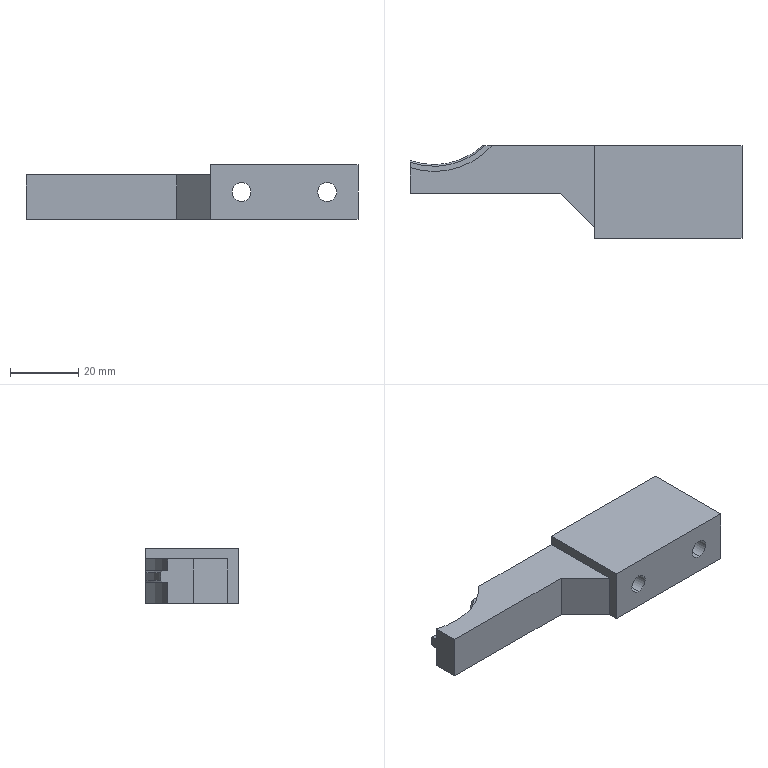Part | SolidWorks | features ICE 9, Chamfer 2, Cut 1, Extrusion 1, Fillet 1, HoleWzd 1, MirrorPattern 1, RefAxis 1 | 1 solid | 27 faces | box 97 x 27 x 16 mm | volume 25539 mm3 | plane 14 | cylinder 11 | cone 2 | commonest cylinder face diameters 5.5 x4 10 x4 46 x2 42 x1
STEP:
#1=CARTESIAN_POINT('',(23.5,14.1,-3.5));
#2=VERTEX_POINT('',#1);
#3=CARTESIAN_POINT('',(23.5,14.1,6.5));
#4=VERTEX_POINT('',#3);
#5=CARTESIAN_POINT('',(23.5,14.1,1.5));
#6=DIRECTION('',(0.,1.,0.));
#7=DIRECTION('',(0.,0.,1.));
#8=AXIS2_PLACEMENT_3D('',#5,#6,#7);
#9=CIRCLE('',#8,5.);
#10=EDGE_CURVE('',#2,#4,#9,.T.);
#11=ORIENTED_EDGE('',*,*,#10,.F.);
#12=CARTESIAN_POINT('',(23.5,19.5,-3.5));
#13=VERTEX_POINT('',#12);
#14=CARTESIAN_POINT('',(23.5,19.5,-3.5));
#15=DIRECTION('',(0.,1.,0.));
#16=VECTOR('',#15,1000.);
#17=LINE('',#14,#16);
#18=EDGE_CURVE('',#2,#13,#17,.T.);
#19=ORIENTED_EDGE('',*,*,#18,.T.);
#20=CARTESIAN_POINT('',(23.5,19.5,6.5));
#21=VERTEX_POINT('',#20);
#22=CARTESIAN_POINT('',(23.5,19.5,1.5));
#23=DIRECTION('',(0.,1.,0.));
#24=DIRECTION('',(0.,0.,1.));
#25=AXIS2_PLACEMENT_3D('',#22,#23,#24);
#26=CIRCLE('',#25,5.);
#27=EDGE_CURVE('',#13,#21,#26,.T.);
#28=ORIENTED_EDGE('',*,*,#27,.T.);
#29=CARTESIAN_POINT('',(23.5,19.5,6.5));
#30=DIRECTION('',(0.,1.,0.));
#31=VECTOR('',#30,1000.);
#32=LINE('',#29,#31);
#33=EDGE_CURVE('',#4,#21,#32,.T.);
#34=ORIENTED_EDGE('',*,*,#33,.F.);
#35=EDGE_LOOP('',(#11,#19,#28,#34));
#36=FACE_OUTER_BOUND('',#35,.T.);
#37=CARTESIAN_POINT('',(23.5,19.5,1.5));
#38=DIRECTION('',(0.,1.,0.));
#39=DIRECTION('',(0.,0.,1.));
#40=AXIS2_PLACEMENT_3D('',#37,#38,#39);
#41=CYLINDRICAL_SURFACE('',#40,5.);
#42=ADVANCED_FACE('',(#36),#41,.F.);
#43=CARTESIAN_POINT('',(23.5,-7.5,-1.25));
#44=VERTEX_POINT('',#43);
#45=CARTESIAN_POINT('',(23.5,-7.5,4.25));
#46=VERTEX_POINT('',#45);
#47=CARTESIAN_POINT('',(23.5,-7.5,1.5));
#48=DIRECTION('',(0.,1.,0.));
#49=DIRECTION('',(0.,0.,1.));
#50=AXIS2_PLACEMENT_3D('',#47,#48,#49);
#51=CIRCLE('',#50,2.75);
#52=EDGE_CURVE('',#44,#46,#51,.T.);
#53=ORIENTED_EDGE('',*,*,#52,.F.);
#54=CARTESIAN_POINT('',(23.5,14.1,-1.25));
#55=VERTEX_POINT('',#54);
#56=CARTESIAN_POINT('',(23.5,19.5,-1.25));
#57=DIRECTION('',(0.,1.,0.));
#58=VECTOR('',#57,1000.);
#59=LINE('',#56,#58);
#60=EDGE_CURVE('',#44,#55,#59,.T.);
#61=ORIENTED_EDGE('',*,*,#60,.T.);
#62=CARTESIAN_POINT('',(23.5,14.1,4.25));
#63=VERTEX_POINT('',#62);
#64=CARTESIAN_POINT('',(23.5,14.1,1.5));
#65=DIRECTION('',(0.,1.,0.));
#66=DIRECTION('',(0.,0.,1.));
#67=AXIS2_PLACEMENT_3D('',#64,#65,#66);
#68=CIRCLE('',#67,2.75);
#69=EDGE_CURVE('',#55,#63,#68,.T.);
#70=ORIENTED_EDGE('',*,*,#69,.T.);
#71=CARTESIAN_POINT('',(23.5,19.5,4.25));
#72=DIRECTION('',(0.,1.,0.));
#73=VECTOR('',#72,1000.);
#74=LINE('',#71,#73);
#75=EDGE_CURVE('',#46,#63,#74,.T.);
#76=ORIENTED_EDGE('',*,*,#75,.F.);
#77=EDGE_LOOP('',(#53,#61,#70,#76));
#78=FACE_OUTER_BOUND('',#77,.T.);
#79=CARTESIAN_POINT('',(23.5,19.5,1.5));
#80=DIRECTION('',(0.,1.,0.));
#81=DIRECTION('',(0.,0.,1.));
#82=AXIS2_PLACEMENT_3D('',#79,#80,#81);
#83=CYLINDRICAL_SURFACE('',#82,2.75);
#84=ADVANCED_FACE('',(#78),#83,.F.);
#85=CARTESIAN_POINT('',(48.5,14.1,-3.5));
#86=VERTEX_POINT('',#85);
#87=CARTESIAN_POINT('',(48.5,14.1,6.5));
#88=VERTEX_POINT('',#87);
#89=CARTESIAN_POINT('',(48.5,14.1,1.5));
#90=DIRECTION('',(0.,1.,0.));
#91=DIRECTION('',(0.,0.,1.));
#92=AXIS2_PLACEMENT_3D('',#89,#90,#91);
#93=CIRCLE('',#92,5.);
#94=EDGE_CURVE('',#86,#88,#93,.T.);
#95=ORIENTED_EDGE('',*,*,#94,.F.);
#96=CARTESIAN_POINT('',(48.5,19.5,-3.5));
#97=VERTEX_POINT('',#96);
#98=CARTESIAN_POINT('',(48.5,19.5,-3.5));
#99=DIRECTION('',(0.,1.,0.));
#100=VECTOR('',#99,1000.);
#101=LINE('',#98,#100);
#102=EDGE_CURVE('',#86,#97,#101,.T.);
#103=ORIENTED_EDGE('',*,*,#102,.T.);
#104=CARTESIAN_POINT('',(48.5,19.5,6.5));
#105=VERTEX_POINT('',#104);
#106=CARTESIAN_POINT('',(48.5,19.5,1.5));
#107=DIRECTION('',(0.,1.,0.));
#108=DIRECTION('',(0.,0.,1.));
#109=AXIS2_PLACEMENT_3D('',#106,#107,#108);
#110=CIRCLE('',#109,5.);
#111=EDGE_CURVE('',#97,#105,#110,.T.);
#112=ORIENTED_EDGE('',*,*,#111,.T.);
#113=CARTESIAN_POINT('',(48.5,19.5,6.5));
#114=DIRECTION('',(0.,1.,0.));
#115=VECTOR('',#114,1000.);
#116=LINE('',#113,#115);
#117=EDGE_CURVE('',#88,#105,#116,.T.);
#118=ORIENTED_EDGE('',*,*,#117,.F.);
#119=EDGE_LOOP('',(#95,#103,#112,#118));
#120=FACE_OUTER_BOUND('',#119,.T.);
#121=CARTESIAN_POINT('',(48.5,19.5,1.5));
#122=DIRECTION('',(0.,1.,0.));
#123=DIRECTION('',(0.,0.,1.));
#124=AXIS2_PLACEMENT_3D('',#121,#122,#123);
#125=CYLINDRICAL_SURFACE('',#124,5.);
#126=ADVANCED_FACE('',(#120),#125,.F.);
#127=CARTESIAN_POINT('',(48.5,-7.5,-1.25));
#128=VERTEX_POINT('',#127);
#129=CARTESIAN_POINT('',(48.5,-7.5,4.25));
#130=VERTEX_POINT('',#129);
#131=CARTESIAN_POINT('',(48.5,-7.5,1.5));
#132=DIRECTION('',(0.,1.,0.));
#133=DIRECTION('',(0.,0.,1.));
#134=AXIS2_PLACEMENT_3D('',#131,#132,#133);
#135=CIRCLE('',#134,2.75);
#136=EDGE_CURVE('',#128,#130,#135,.T.);
#137=ORIENTED_EDGE('',*,*,#136,.F.);
#138=CARTESIAN_POINT('',(48.5,14.1,-1.25));
#139=VERTEX_POINT('',#138);
#140=CARTESIAN_POINT('',(48.5,19.5,-1.25));
#141=DIRECTION('',(0.,1.,0.));
#142=VECTOR('',#141,1000.);
#143=LINE('',#140,#142);
#144=EDGE_CURVE('',#128,#139,#143,.T.);
#145=ORIENTED_EDGE('',*,*,#144,.T.);
#146=CARTESIAN_POINT('',(48.5,14.1,4.25));
#147=VERTEX_POINT('',#146);
#148=CARTESIAN_POINT('',(48.5,14.1,1.5));
#149=DIRECTION('',(0.,1.,0.));
#150=DIRECTION('',(0.,0.,1.));
#151=AXIS2_PLACEMENT_3D('',#148,#149,#150);
#152=CIRCLE('',#151,2.75);
#153=EDGE_CURVE('',#139,#147,#152,.T.);
#154=ORIENTED_EDGE('',*,*,#153,.T.);
#155=CARTESIAN_POINT('',(48.5,19.5,4.25));
#156=DIRECTION('',(0.,1.,0.));
#157=VECTOR('',#156,1000.);
#158=LINE('',#155,#157);
#159=EDGE_CURVE('',#130,#147,#158,.T.);
#160=ORIENTED_EDGE('',*,*,#159,.F.);
#161=EDGE_LOOP('',(#137,#145,#154,#160));
#162=FACE_OUTER_BOUND('',#161,.T.);
#163=CARTESIAN_POINT('',(48.5,19.5,1.5));
#164=DIRECTION('',(0.,1.,0.));
#165=DIRECTION('',(0.,0.,1.));
#166=AXIS2_PLACEMENT_3D('',#163,#164,#165);
#167=CYLINDRICAL_SURFACE('',#166,2.75);
#168=ADVANCED_FACE('',(#162),#167,.F.);
#169=CARTESIAN_POINT('',(23.5,19.5,1.5));
#170=DIRECTION('',(0.,1.,0.));
#171=DIRECTION('',(0.,0.,1.));
#172=AXIS2_PLACEMENT_3D('',#169,#170,#171);
#173=CIRCLE('',#172,5.);
#174=EDGE_CURVE('',#21,#13,#173,.T.);
#175=ORIENTED_EDGE('',*,*,#174,.F.);
#176=ORIENTED_EDGE('',*,*,#27,.F.);
#177=EDGE_LOOP('',(#175,#176));
#178=FACE_BOUND('',#177,.T.);
#179=CARTESIAN_POINT('',(-15.507,19.5,-0.3));
#180=VERTEX_POINT('',#179);
#181=CARTESIAN_POINT('',(-17.6,19.5,-0.3));
#182=VERTEX_POINT('',#181);
#183=CARTESIAN_POINT('',(-32.5,19.5,-0.3));
#184=DIRECTION('',(-1.,0.,0.));
#185=VECTOR('',#184,1000.);
#186=LINE('',#183,#185);
#187=EDGE_CURVE('',#180,#182,#186,.T.);
#188=ORIENTED_EDGE('',*,*,#187,.T.);
#189=CARTESIAN_POINT('',(-18.331,19.5,0.2));
#190=VERTEX_POINT('',#189);
#191=CARTESIAN_POINT('',(-17.6,19.5,-0.3));
#192=CARTESIAN_POINT('',(-17.843,19.5,-0.1317));
#193=CARTESIAN_POINT('',(-18.087,19.5,0.03503));
#194=CARTESIAN_POINT('',(-18.331,19.5,0.2));
#195=B_SPLINE_CURVE_WITH_KNOTS('',3,(#191,#192,#193,#194),.UNSPECIFIED.,.F.,.F.,(4,4),(0.000001215,0.0008778),.UNSPECIFIED.);
#196=EDGE_CURVE('',#182,#190,#195,.T.);
#197=ORIENTED_EDGE('',*,*,#196,.T.);
#198=CARTESIAN_POINT('',(-18.331,19.5,2.5));
#199=VERTEX_POINT('',#198);
#200=CARTESIAN_POINT('',(-18.331,19.5,-9.5));
#201=DIRECTION('',(0.,0.,-1.));
#202=VECTOR('',#201,1000.);
#203=LINE('',#200,#202);
#204=EDGE_CURVE('',#199,#190,#203,.T.);
#205=ORIENTED_EDGE('',*,*,#204,.F.);
#206=CARTESIAN_POINT('',(-17.6,19.5,3.));
#207=VERTEX_POINT('',#206);
#208=CARTESIAN_POINT('',(-18.331,19.5,2.5));
#209=CARTESIAN_POINT('',(-18.087,19.5,2.665));
#210=CARTESIAN_POINT('',(-17.843,19.5,2.832));
#211=CARTESIAN_POINT('',(-17.6,19.5,3.));
#212=B_SPLINE_CURVE_WITH_KNOTS('',3,(#208,#209,#210,#211),.UNSPECIFIED.,.F.,.F.,(4,4),(0.03127,0.03213),.UNSPECIFIED.);
#213=EDGE_CURVE('',#199,#207,#212,.T.);
#214=ORIENTED_EDGE('',*,*,#213,.T.);
#215=CARTESIAN_POINT('',(-15.507,19.5,3.));
#216=VERTEX_POINT('',#215);
#217=CARTESIAN_POINT('',(-32.5,19.5,3.));
#218=DIRECTION('',(1.,0.,0.));
#219=VECTOR('',#218,1000.);
#220=LINE('',#217,#219);
#221=EDGE_CURVE('',#207,#216,#220,.T.);
#222=ORIENTED_EDGE('',*,*,#221,.T.);
#223=CARTESIAN_POINT('',(-15.507,19.5,6.5));
#224=VERTEX_POINT('',#223);
#225=CARTESIAN_POINT('',(-15.507,19.5,3.));
#226=DIRECTION('',(0.,0.,-1.));
#227=VECTOR('',#226,1000.);
#228=LINE('',#225,#227);
#229=EDGE_CURVE('',#224,#216,#228,.T.);
#230=ORIENTED_EDGE('',*,*,#229,.F.);
#231=CARTESIAN_POINT('',(14.5,19.5,6.5));
#232=VERTEX_POINT('',#231);
#233=CARTESIAN_POINT('',(0.,19.5,6.5));
#234=DIRECTION('',(1.,0.,0.));
#235=VECTOR('',#234,1000.);
#236=LINE('',#233,#235);
#237=EDGE_CURVE('',#224,#232,#236,.T.);
#238=ORIENTED_EDGE('',*,*,#237,.T.);
#239=CARTESIAN_POINT('',(14.5,19.5,9.5));
#240=VERTEX_POINT('',#239);
#241=CARTESIAN_POINT('',(14.5,19.5,6.5));
#242=DIRECTION('',(0.,0.,-1.));
#243=VECTOR('',#242,1000.);
#244=LINE('',#241,#243);
#245=EDGE_CURVE('',#240,#232,#244,.T.);
#246=ORIENTED_EDGE('',*,*,#245,.F.);
#247=CARTESIAN_POINT('',(57.5,19.5,9.5));
#248=VERTEX_POINT('',#247);
#249=CARTESIAN_POINT('',(57.5,19.5,9.5));
#250=DIRECTION('',(1.,0.,0.));
#251=VECTOR('',#250,1000.);
#252=LINE('',#249,#251);
#253=EDGE_CURVE('',#240,#248,#252,.T.);
#254=ORIENTED_EDGE('',*,*,#253,.T.);
#255=CARTESIAN_POINT('',(57.5,19.5,-6.5));
#256=VERTEX_POINT('',#255);
#257=CARTESIAN_POINT('',(57.5,19.5,-6.5));
#258=DIRECTION('',(0.,0.,1.));
#259=VECTOR('',#258,1000.);
#260=LINE('',#257,#259);
#261=EDGE_CURVE('',#256,#248,#260,.T.);
#262=ORIENTED_EDGE('',*,*,#261,.F.);
#263=CARTESIAN_POINT('',(-15.507,19.5,-6.5));
#264=VERTEX_POINT('',#263);
#265=CARTESIAN_POINT('',(0.,19.5,-6.5));
#266=DIRECTION('',(-1.,0.,0.));
#267=VECTOR('',#266,1000.);
#268=LINE('',#265,#267);
#269=EDGE_CURVE('',#256,#264,#268,.T.);
#270=ORIENTED_EDGE('',*,*,#269,.T.);
#271=CARTESIAN_POINT('',(-15.507,19.5,-0.3));
#272=DIRECTION('',(0.,0.,-1.));
#273=VECTOR('',#272,1000.);
#274=LINE('',#271,#273);
#275=EDGE_CURVE('',#180,#264,#274,.T.);
#276=ORIENTED_EDGE('',*,*,#275,.F.);
#277=EDGE_LOOP('',(#188,#197,#205,#214,#222,#230,#238,#246,#254,#262,#270,#276));
#278=FACE_OUTER_BOUND('',#277,.T.);
#279=CARTESIAN_POINT('',(48.5,19.5,1.5));
#280=DIRECTION('',(0.,1.,0.));
#281=DIRECTION('',(0.,0.,1.));
#282=AXIS2_PLACEMENT_3D('',#279,#280,#281);
#283=CIRCLE('',#282,5.);
#284=EDGE_CURVE('',#105,#97,#283,.T.);
#285=ORIENTED_EDGE('',*,*,#284,.F.);
#286=ORIENTED_EDGE('',*,*,#111,.F.);
#287=EDGE_LOOP('',(#285,#286));
#288=FACE_BOUND('',#287,.T.);
#289=CARTESIAN_POINT('',(57.5,19.5,-6.5));
#290=DIRECTION('',(0.,-1.,0.));
#291=DIRECTION('',(1.,0.,0.));
#292=AXIS2_PLACEMENT_3D('',#289,#290,#291);
#293=PLANE('',#292);
#294=ADVANCED_FACE('',(#178,#278,#288),#293,.F.);
#295=CARTESIAN_POINT('',(23.5,-7.5,1.5));
#296=DIRECTION('',(0.,1.,0.));
#297=DIRECTION('',(0.,0.,1.));
#298=AXIS2_PLACEMENT_3D('',#295,#296,#297);
#299=CIRCLE('',#298,2.75);
#300=EDGE_CURVE('',#46,#44,#299,.T.);
#301=ORIENTED_EDGE('',*,*,#300,.T.);
#302=ORIENTED_EDGE('',*,*,#52,.T.);
#303=EDGE_LOOP('',(#301,#302));
#304=FACE_BOUND('',#303,.T.);
#305=CARTESIAN_POINT('',(48.5,-7.5,1.5));
#306=DIRECTION('',(0.,1.,0.));
#307=DIRECTION('',(0.,0.,1.));
#308=AXIS2_PLACEMENT_3D('',#305,#306,#307);
#309=CIRCLE('',#308,2.75);
#310=EDGE_CURVE('',#130,#128,#309,.T.);
#311=ORIENTED_EDGE('',*,*,#310,.T.);
#312=ORIENTED_EDGE('',*,*,#136,.T.);
#313=EDGE_LOOP('',(#311,#312));
#314=FACE_BOUND('',#313,.T.);
#315=CARTESIAN_POINT('',(14.5,-7.5,-6.5));
#316=VERTEX_POINT('',#315);
#317=CARTESIAN_POINT('',(14.5,-7.5,9.5));
#318=VERTEX_POINT('',#317);
#319=CARTESIAN_POINT('',(14.5,-7.5,6.5));
#320=DIRECTION('',(0.,0.,1.));
#321=VECTOR('',#320,1000.);
#322=LINE('',#319,#321);
#323=EDGE_CURVE('',#316,#318,#322,.T.);
#324=ORIENTED_EDGE('',*,*,#323,.F.);
#325=CARTESIAN_POINT('',(57.5,-7.5,-6.5));
#326=VERTEX_POINT('',#325);
#327=CARTESIAN_POINT('',(14.5,-7.5,-6.5));
#328=DIRECTION('',(1.,0.,0.));
#329=VECTOR('',#328,1000.);
#330=LINE('',#327,#329);
#331=EDGE_CURVE('',#316,#326,#330,.T.);
#332=ORIENTED_EDGE('',*,*,#331,.T.);
#333=CARTESIAN_POINT('',(57.5,-7.5,9.5));
#334=VERTEX_POINT('',#333);
#335=CARTESIAN_POINT('',(57.5,-7.5,-9.5));
#336=DIRECTION('',(0.,0.,-1.));
#337=VECTOR('',#336,1000.);
#338=LINE('',#335,#337);
#339=EDGE_CURVE('',#334,#326,#338,.T.);
#340=ORIENTED_EDGE('',*,*,#339,.F.);
#341=CARTESIAN_POINT('',(-57.5,-7.5,9.5));
#342=DIRECTION('',(1.,0.,0.));
#343=VECTOR('',#342,1000.);
#344=LINE('',#341,#343);
#345=EDGE_CURVE('',#318,#334,#344,.T.);
#346=ORIENTED_EDGE('',*,*,#345,.F.);
#347=EDGE_LOOP('',(#324,#332,#340,#346));
#348=FACE_OUTER_BOUND('',#347,.T.);
#349=CARTESIAN_POINT('',(0.,-7.5,0.));
#350=DIRECTION('',(0.,1.,0.));
#351=DIRECTION('',(0.,0.,1.));
#352=AXIS2_PLACEMENT_3D('',#349,#350,#351);
#353=PLANE('',#352);
#354=ADVANCED_FACE('',(#304,#314,#348),#353,.F.);
#355=CARTESIAN_POINT('',(-39.5,13.091,-6.5));
#356=VERTEX_POINT('',#355);
#357=CARTESIAN_POINT('',(-32.5,35.,-6.5));
#358=DIRECTION('',(0.,0.,1.));
#359=DIRECTION('',(-1.,0.,0.));
#360=AXIS2_PLACEMENT_3D('',#357,#358,#359);
#361=CIRCLE('',#360,23.);
#362=EDGE_CURVE('',#356,#264,#361,.T.);
#363=ORIENTED_EDGE('',*,*,#362,.F.);
#364=CARTESIAN_POINT('',(-39.5,13.091,-0.3));
#365=VERTEX_POINT('',#364);
#366=CARTESIAN_POINT('',(-39.5,13.091,-0.3));
#367=DIRECTION('',(0.,0.,1.));
#368=VECTOR('',#367,1000.);
#369=LINE('',#366,#368);
#370=EDGE_CURVE('',#356,#365,#369,.T.);
#371=ORIENTED_EDGE('',*,*,#370,.T.);
#372=CARTESIAN_POINT('',(-32.5,35.,-0.3));
#373=DIRECTION('',(0.,0.,-1.));
#374=DIRECTION('',(-1.,0.,0.));
#375=AXIS2_PLACEMENT_3D('',#372,#373,#374);
#376=CIRCLE('',#375,23.);
#377=EDGE_CURVE('',#180,#365,#376,.T.);
#378=ORIENTED_EDGE('',*,*,#377,.F.);
#379=ORIENTED_EDGE('',*,*,#275,.T.);
#380=EDGE_LOOP('',(#363,#371,#378,#379));
#381=FACE_OUTER_BOUND('',#380,.T.);
#382=CARTESIAN_POINT('',(-32.5,35.,-0.3));
#383=DIRECTION('',(0.,0.,-1.));
#384=DIRECTION('',(-1.,0.,0.));
#385=AXIS2_PLACEMENT_3D('',#382,#383,#384);
#386=CYLINDRICAL_SURFACE('',#385,23.);
#387=ADVANCED_FACE('',(#381),#386,.F.);
#388=CARTESIAN_POINT('',(-39.5,13.091,3.));
#389=VERTEX_POINT('',#388);
#390=CARTESIAN_POINT('',(-32.5,35.,3.));
#391=DIRECTION('',(0.,0.,1.));
#392=DIRECTION('',(1.,0.,0.));
#393=AXIS2_PLACEMENT_3D('',#390,#391,#392);
#394=CIRCLE('',#393,23.);
#395=EDGE_CURVE('',#389,#216,#394,.T.);
#396=ORIENTED_EDGE('',*,*,#395,.F.);
#397=CARTESIAN_POINT('',(-39.5,13.091,6.5));
#398=VERTEX_POINT('',#397);
#399=CARTESIAN_POINT('',(-39.5,13.091,3.));
#400=DIRECTION('',(0.,0.,1.));
#401=VECTOR('',#400,1000.);
#402=LINE('',#399,#401);
#403=EDGE_CURVE('',#389,#398,#402,.T.);
#404=ORIENTED_EDGE('',*,*,#403,.T.);
#405=CARTESIAN_POINT('',(-32.5,35.,6.5));
#406=DIRECTION('',(0.,0.,-1.));
#407=DIRECTION('',(1.,0.,0.));
#408=AXIS2_PLACEMENT_3D('',#405,#406,#407);
#409=CIRCLE('',#408,23.);
#410=EDGE_CURVE('',#224,#398,#409,.T.);
#411=ORIENTED_EDGE('',*,*,#410,.F.);
#412=ORIENTED_EDGE('',*,*,#229,.T.);
#413=EDGE_LOOP('',(#396,#404,#411,#412));
#414=FACE_OUTER_BOUND('',#413,.T.);
#415=CARTESIAN_POINT('',(-32.5,35.,3.));
#416=DIRECTION('',(0.,0.,1.));
#417=DIRECTION('',(1.,0.,0.));
#418=AXIS2_PLACEMENT_3D('',#415,#416,#417);
#419=CYLINDRICAL_SURFACE('',#418,23.);
#420=ADVANCED_FACE('',(#414),#419,.F.);
#421=CARTESIAN_POINT('',(57.5,-7.5,-6.5));
#422=DIRECTION('',(0.,1.,0.));
#423=VECTOR('',#422,1000.);
#424=LINE('',#421,#423);
#425=EDGE_CURVE('',#326,#256,#424,.T.);
#426=ORIENTED_EDGE('',*,*,#425,.T.);
#427=ORIENTED_EDGE('',*,*,#261,.T.);
#428=CARTESIAN_POINT('',(57.5,7.5,9.5));
#429=DIRECTION('',(0.,-1.,0.));
#430=VECTOR('',#429,1000.);
#431=LINE('',#428,#430);
#432=EDGE_CURVE('',#248,#334,#431,.T.);
#433=ORIENTED_EDGE('',*,*,#432,.T.);
#434=ORIENTED_EDGE('',*,*,#339,.T.);
#435=EDGE_LOOP('',(#426,#427,#433,#434));
#436=FACE_OUTER_BOUND('',#435,.T.);
#437=CARTESIAN_POINT('',(57.5,7.5,-9.5));
#438=DIRECTION('',(-1.,0.,0.));
#439=DIRECTION('',(0.,0.,1.));
#440=AXIS2_PLACEMENT_3D('',#437,#438,#439);
#441=PLANE('',#440);
#442=ADVANCED_FACE('',(#436),#441,.F.);
#443=ORIENTED_EDGE('',*,*,#432,.F.);
#444=ORIENTED_EDGE('',*,*,#253,.F.);
#445=CARTESIAN_POINT('',(14.5,-7.5,9.5));
#446=DIRECTION('',(0.,1.,0.));
#447=VECTOR('',#446,1000.);
#448=LINE('',#445,#447);
#449=EDGE_CURVE('',#318,#240,#448,.T.);
#450=ORIENTED_EDGE('',*,*,#449,.F.);
#451=ORIENTED_EDGE('',*,*,#345,.T.);
#452=EDGE_LOOP('',(#443,#444,#450,#451));
#453=FACE_OUTER_BOUND('',#452,.T.);
#454=CARTESIAN_POINT('',(-57.5,7.5,9.5));
#455=DIRECTION('',(0.,0.,-1.));
#456=DIRECTION('',(-1.,0.,0.));
#457=AXIS2_PLACEMENT_3D('',#454,#455,#456);
#458=PLANE('',#457);
#459=ADVANCED_FACE('',(#453),#458,.F.);
#460=CARTESIAN_POINT('',(-39.5,14.671,3.));
#461=VERTEX_POINT('',#460);
#462=CARTESIAN_POINT('',(-39.5,35.,3.));
#463=DIRECTION('',(0.,1.,0.));
#464=VECTOR('',#463,1000.);
#465=LINE('',#462,#464);
#466=EDGE_CURVE('',#389,#461,#465,.T.);
#467=ORIENTED_EDGE('',*,*,#466,.F.);
#468=ORIENTED_EDGE('',*,*,#395,.T.);
#469=ORIENTED_EDGE('',*,*,#221,.F.);
#470=CARTESIAN_POINT('',(-32.5,35.,3.));
#471=DIRECTION('',(0.,0.,-1.));
#472=DIRECTION('',(1.,0.,0.));
#473=AXIS2_PLACEMENT_3D('',#470,#471,#472);
#474=CIRCLE('',#473,21.5);
#475=EDGE_CURVE('',#207,#461,#474,.T.);
#476=ORIENTED_EDGE('',*,*,#475,.T.);
#477=EDGE_LOOP('',(#467,#468,#469,#476));
#478=FACE_OUTER_BOUND('',#477,.T.);
#479=CARTESIAN_POINT('',(-32.5,35.,3.));
#480=DIRECTION('',(0.,0.,1.));
#481=DIRECTION('',(1.,0.,0.));
#482=AXIS2_PLACEMENT_3D('',#479,#480,#481);
#483=PLANE('',#482);
#484=ADVANCED_FACE('',(#478),#483,.T.);
#485=CARTESIAN_POINT('',(-39.5,14.671,-0.3));
#486=VERTEX_POINT('',#485);
#487=CARTESIAN_POINT('',(-39.5,35.,-0.3));
#488=DIRECTION('',(0.,-1.,0.));
#489=VECTOR('',#488,1000.);
#490=LINE('',#487,#489);
#491=EDGE_CURVE('',#486,#365,#490,.T.);
#492=ORIENTED_EDGE('',*,*,#491,.F.);
#493=CARTESIAN_POINT('',(-32.5,35.,-0.3));
#494=DIRECTION('',(0.,0.,1.));
#495=DIRECTION('',(-1.,0.,0.));
#496=AXIS2_PLACEMENT_3D('',#493,#494,#495);
#497=CIRCLE('',#496,21.5);
#498=EDGE_CURVE('',#486,#182,#497,.T.);
#499=ORIENTED_EDGE('',*,*,#498,.T.);
#500=ORIENTED_EDGE('',*,*,#187,.F.);
#501=ORIENTED_EDGE('',*,*,#377,.T.);
#502=EDGE_LOOP('',(#492,#499,#500,#501));
#503=FACE_OUTER_BOUND('',#502,.T.);
#504=CARTESIAN_POINT('',(-32.5,35.,-0.3));
#505=DIRECTION('',(0.,0.,-1.));
#506=DIRECTION('',(-1.,0.,0.));
#507=AXIS2_PLACEMENT_3D('',#504,#505,#506);
#508=PLANE('',#507);
#509=ADVANCED_FACE('',(#503),#508,.T.);
#510=CARTESIAN_POINT('',(-39.5,15.201,0.2));
#511=VERTEX_POINT('',#510);
#512=CARTESIAN_POINT('',(-32.5,35.,0.2));
#513=DIRECTION('',(0.,0.,-1.));
#514=DIRECTION('',(-1.,0.,0.));
#515=AXIS2_PLACEMENT_3D('',#512,#513,#514);
#516=CIRCLE('',#515,21.);
#517=EDGE_CURVE('',#190,#511,#516,.T.);
#518=ORIENTED_EDGE('',*,*,#517,.T.);
#519=CARTESIAN_POINT('',(-39.5,15.201,2.5));
#520=VERTEX_POINT('',#519);
#521=CARTESIAN_POINT('',(-39.5,15.201,-9.5));
#522=DIRECTION('',(0.,0.,1.));
#523=VECTOR('',#522,1000.);
#524=LINE('',#521,#523);
#525=EDGE_CURVE('',#511,#520,#524,.T.);
#526=ORIENTED_EDGE('',*,*,#525,.T.);
#527=CARTESIAN_POINT('',(-32.5,35.,2.5));
#528=DIRECTION('',(0.,0.,1.));
#529=DIRECTION('',(1.,0.,0.));
#530=AXIS2_PLACEMENT_3D('',#527,#528,#529);
#531=CIRCLE('',#530,21.);
#532=EDGE_CURVE('',#520,#199,#531,.T.);
#533=ORIENTED_EDGE('',*,*,#532,.T.);
#534=ORIENTED_EDGE('',*,*,#204,.T.);
#535=EDGE_LOOP('',(#518,#526,#533,#534));
#536=FACE_OUTER_BOUND('',#535,.T.);
#537=CARTESIAN_POINT('',(-32.5,35.,-9.5));
#538=DIRECTION('',(0.,0.,1.));
#539=DIRECTION('',(1.,0.,0.));
#540=AXIS2_PLACEMENT_3D('',#537,#538,#539);
#541=CYLINDRICAL_SURFACE('',#540,21.);
#542=ADVANCED_FACE('',(#536),#541,.F.);
#543=CARTESIAN_POINT('',(-39.5,15.201,0.2));
#544=CARTESIAN_POINT('',(-39.5,15.024,0.03346));
#545=CARTESIAN_POINT('',(-39.5,14.848,-0.1332));
#546=CARTESIAN_POINT('',(-39.5,14.671,-0.3));
#547=B_SPLINE_CURVE_WITH_KNOTS('',3,(#543,#544,#545,#546),.UNSPECIFIED.,.F.,.F.,(4,4),(0.008901,0.009629),.UNSPECIFIED.);
#548=EDGE_CURVE('',#511,#486,#547,.T.);
#549=ORIENTED_EDGE('',*,*,#548,.F.);
#550=ORIENTED_EDGE('',*,*,#517,.F.);
#551=ORIENTED_EDGE('',*,*,#196,.F.);
#552=ORIENTED_EDGE('',*,*,#498,.F.);
#553=EDGE_LOOP('',(#549,#550,#551,#552));
#554=FACE_OUTER_BOUND('',#553,.T.);
#555=CARTESIAN_POINT('',(-32.5,35.,0.2));
#556=DIRECTION('',(0.,0.,-1.));
#557=DIRECTION('',(-1.,0.,0.));
#558=AXIS2_PLACEMENT_3D('',#555,#556,#557);
#559=CONICAL_SURFACE('',#558,21.,0.7854);
#560=ADVANCED_FACE('',(#554),#559,.F.);
#561=CARTESIAN_POINT('',(-39.5,14.671,3.));
#562=CARTESIAN_POINT('',(-39.5,14.848,2.833));
#563=CARTESIAN_POINT('',(-39.5,15.024,2.667));
#564=CARTESIAN_POINT('',(-39.5,15.201,2.5));
#565=B_SPLINE_CURVE_WITH_KNOTS('',3,(#561,#562,#563,#564),.UNSPECIFIED.,.F.,.F.,(4,4),(0.008705,0.009433),.UNSPECIFIED.);
#566=EDGE_CURVE('',#461,#520,#565,.T.);
#567=ORIENTED_EDGE('',*,*,#566,.F.);
#568=ORIENTED_EDGE('',*,*,#475,.F.);
#569=ORIENTED_EDGE('',*,*,#213,.F.);
#570=ORIENTED_EDGE('',*,*,#532,.F.);
#571=EDGE_LOOP('',(#567,#568,#569,#570));
#572=FACE_OUTER_BOUND('',#571,.T.);
#573=CARTESIAN_POINT('',(-32.5,35.,2.5));
#574=DIRECTION('',(0.,0.,1.));
#575=DIRECTION('',(1.,0.,0.));
#576=AXIS2_PLACEMENT_3D('',#573,#574,#575);
#577=CONICAL_SURFACE('',#576,21.,0.7854);
#578=ADVANCED_FACE('',(#572),#577,.F.);
#579=CARTESIAN_POINT('',(-39.5,5.5,6.5));
#580=VERTEX_POINT('',#579);
#581=CARTESIAN_POINT('',(-39.5,0.,6.5));
#582=DIRECTION('',(0.,1.,0.));
#583=VECTOR('',#582,1000.);
#584=LINE('',#581,#583);
#585=EDGE_CURVE('',#580,#398,#584,.T.);
#586=ORIENTED_EDGE('',*,*,#585,.F.);
#587=CARTESIAN_POINT('',(4.5,5.5,6.5));
#588=VERTEX_POINT('',#587);
#589=CARTESIAN_POINT('',(-57.5,5.5,6.5));
#590=DIRECTION('',(-1.,0.,0.));
#591=VECTOR('',#590,1000.);
#592=LINE('',#589,#591);
#593=EDGE_CURVE('',#588,#580,#592,.T.);
#594=ORIENTED_EDGE('',*,*,#593,.F.);
#595=CARTESIAN_POINT('',(14.5,-4.5,6.5));
#596=VERTEX_POINT('',#595);
#597=CARTESIAN_POINT('',(4.5,5.5,6.5));
#598=DIRECTION('',(0.7071,-0.7071,0.));
#599=VECTOR('',#598,1000.);
#600=LINE('',#597,#599);
#601=EDGE_CURVE('',#588,#596,#600,.T.);
#602=ORIENTED_EDGE('',*,*,#601,.T.);
#603=CARTESIAN_POINT('',(14.5,-7.5,6.5));
#604=DIRECTION('',(0.,1.,0.));
#605=VECTOR('',#604,1000.);
#606=LINE('',#603,#605);
#607=EDGE_CURVE('',#596,#232,#606,.T.);
#608=ORIENTED_EDGE('',*,*,#607,.T.);
#609=ORIENTED_EDGE('',*,*,#237,.F.);
#610=ORIENTED_EDGE('',*,*,#410,.T.);
#611=EDGE_LOOP('',(#586,#594,#602,#608,#609,#610));
#612=FACE_OUTER_BOUND('',#611,.T.);
#613=CARTESIAN_POINT('',(0.,0.,6.5));
#614=DIRECTION('',(0.,0.,1.));
#615=DIRECTION('',(1.,0.,0.));
#616=AXIS2_PLACEMENT_3D('',#613,#614,#615);
#617=PLANE('',#616);
#618=ADVANCED_FACE('',(#612),#617,.T.);
#619=ORIENTED_EDGE('',*,*,#607,.F.);
#620=CARTESIAN_POINT('',(14.5,-4.5,-6.5));
#621=VERTEX_POINT('',#620);
#622=CARTESIAN_POINT('',(14.5,-4.5,-6.5));
#623=DIRECTION('',(0.,0.,-1.));
#624=VECTOR('',#623,1000.);
#625=LINE('',#622,#624);
#626=EDGE_CURVE('',#596,#621,#625,.T.);
#627=ORIENTED_EDGE('',*,*,#626,.T.);
#628=CARTESIAN_POINT('',(14.5,-7.5,-6.5));
#629=DIRECTION('',(0.,1.,0.));
#630=VECTOR('',#629,1000.);
#631=LINE('',#628,#630);
#632=EDGE_CURVE('',#316,#621,#631,.T.);
#633=ORIENTED_EDGE('',*,*,#632,.F.);
#634=ORIENTED_EDGE('',*,*,#323,.T.);
#635=ORIENTED_EDGE('',*,*,#449,.T.);
#636=ORIENTED_EDGE('',*,*,#245,.T.);
#637=EDGE_LOOP('',(#619,#627,#633,#634,#635,#636));
#638=FACE_OUTER_BOUND('',#637,.T.);
#639=CARTESIAN_POINT('',(14.5,-7.5,6.5));
#640=DIRECTION('',(1.,0.,0.));
#641=DIRECTION('',(0.,0.,-1.));
#642=AXIS2_PLACEMENT_3D('',#639,#640,#641);
#643=PLANE('',#642);
#644=ADVANCED_FACE('',(#638),#643,.F.);
#645=CARTESIAN_POINT('',(-39.5,5.5,-6.5));
#646=VERTEX_POINT('',#645);
#647=CARTESIAN_POINT('',(-39.5,27.323,-6.5));
#648=DIRECTION('',(0.,-1.,0.));
#649=VECTOR('',#648,1000.);
#650=LINE('',#647,#649);
#651=EDGE_CURVE('',#356,#646,#650,.T.);
#652=ORIENTED_EDGE('',*,*,#651,.F.);
#653=ORIENTED_EDGE('',*,*,#362,.T.);
#654=ORIENTED_EDGE('',*,*,#269,.F.);
#655=ORIENTED_EDGE('',*,*,#425,.F.);
#656=ORIENTED_EDGE('',*,*,#331,.F.);
#657=ORIENTED_EDGE('',*,*,#632,.T.);
#658=CARTESIAN_POINT('',(4.5,5.5,-6.5));
#659=VERTEX_POINT('',#658);
#660=CARTESIAN_POINT('',(4.5,5.5,-6.5));
#661=DIRECTION('',(-0.7071,0.7071,0.));
#662=VECTOR('',#661,1000.);
#663=LINE('',#660,#662);
#664=EDGE_CURVE('',#621,#659,#663,.T.);
#665=ORIENTED_EDGE('',*,*,#664,.T.);
#666=CARTESIAN_POINT('',(-57.5,5.5,-6.5));
#667=DIRECTION('',(-1.,0.,0.));
#668=VECTOR('',#667,1000.);
#669=LINE('',#666,#668);
#670=EDGE_CURVE('',#659,#646,#669,.T.);
#671=ORIENTED_EDGE('',*,*,#670,.T.);
#672=EDGE_LOOP('',(#652,#653,#654,#655,#656,#657,#665,#671));
#673=FACE_OUTER_BOUND('',#672,.T.);
#674=CARTESIAN_POINT('',(0.,0.,-6.5));
#675=DIRECTION('',(0.,0.,-1.));
#676=DIRECTION('',(1.,0.,0.));
#677=AXIS2_PLACEMENT_3D('',#674,#675,#676);
#678=PLANE('',#677);
#679=ADVANCED_FACE('',(#673),#678,.T.);
#680=ORIENTED_EDGE('',*,*,#593,.T.);
#681=CARTESIAN_POINT('',(-39.5,5.5,-6.5));
#682=DIRECTION('',(0.,0.,-1.));
#683=VECTOR('',#682,1000.);
#684=LINE('',#681,#683);
#685=EDGE_CURVE('',#580,#646,#684,.T.);
#686=ORIENTED_EDGE('',*,*,#685,.T.);
#687=ORIENTED_EDGE('',*,*,#670,.F.);
#688=CARTESIAN_POINT('',(4.5,5.5,6.5));
#689=DIRECTION('',(0.,0.,1.));
#690=VECTOR('',#689,1000.);
#691=LINE('',#688,#690);
#692=EDGE_CURVE('',#659,#588,#691,.T.);
#693=ORIENTED_EDGE('',*,*,#692,.T.);
#694=EDGE_LOOP('',(#680,#686,#687,#693));
#695=FACE_OUTER_BOUND('',#694,.T.);
#696=CARTESIAN_POINT('',(-57.5,5.5,-6.5));
#697=DIRECTION('',(0.,1.,0.));
#698=DIRECTION('',(0.,0.,1.));
#699=AXIS2_PLACEMENT_3D('',#696,#697,#698);
#700=PLANE('',#699);
#701=ADVANCED_FACE('',(#695),#700,.F.);
#702=ORIENTED_EDGE('',*,*,#664,.F.);
#703=ORIENTED_EDGE('',*,*,#626,.F.);
#704=ORIENTED_EDGE('',*,*,#601,.F.);
#705=ORIENTED_EDGE('',*,*,#692,.F.);
#706=EDGE_LOOP('',(#702,#703,#704,#705));
#707=FACE_OUTER_BOUND('',#706,.T.);
#708=CARTESIAN_POINT('',(4.5,5.5,-6.5));
#709=DIRECTION('',(-0.7071,-0.7071,0.));
#710=DIRECTION('',(0.,0.,-1.));
#711=AXIS2_PLACEMENT_3D('',#708,#709,#710);
#712=PLANE('',#711);
#713=ADVANCED_FACE('',(#707),#712,.T.);
#714=ORIENTED_EDGE('',*,*,#144,.F.);
#715=ORIENTED_EDGE('',*,*,#310,.F.);
#716=ORIENTED_EDGE('',*,*,#159,.T.);
#717=CARTESIAN_POINT('',(48.5,14.1,1.5));
#718=DIRECTION('',(0.,1.,0.));
#719=DIRECTION('',(0.,0.,1.));
#720=AXIS2_PLACEMENT_3D('',#717,#718,#719);
#721=CIRCLE('',#720,2.75);
#722=EDGE_CURVE('',#147,#139,#721,.T.);
#723=ORIENTED_EDGE('',*,*,#722,.T.);
#724=EDGE_LOOP('',(#714,#715,#716,#723));
#725=FACE_OUTER_BOUND('',#724,.T.);
#726=CARTESIAN_POINT('',(48.5,19.5,1.5));
#727=DIRECTION('',(0.,1.,0.));
#728=DIRECTION('',(0.,0.,1.));
#729=AXIS2_PLACEMENT_3D('',#726,#727,#728);
#730=CYLINDRICAL_SURFACE('',#729,2.75);
#731=ADVANCED_FACE('',(#725),#730,.F.);
#732=ORIENTED_EDGE('',*,*,#722,.F.);
#733=ORIENTED_EDGE('',*,*,#153,.F.);
#734=EDGE_LOOP('',(#732,#733));
#735=FACE_BOUND('',#734,.T.);
#736=CARTESIAN_POINT('',(48.5,14.1,1.5));
#737=DIRECTION('',(0.,1.,0.));
#738=DIRECTION('',(0.,0.,1.));
#739=AXIS2_PLACEMENT_3D('',#736,#737,#738);
#740=CIRCLE('',#739,5.);
#741=EDGE_CURVE('',#88,#86,#740,.T.);
#742=ORIENTED_EDGE('',*,*,#741,.T.);
#743=ORIENTED_EDGE('',*,*,#94,.T.);
#744=EDGE_LOOP('',(#742,#743));
#745=FACE_OUTER_BOUND('',#744,.T.);
#746=CARTESIAN_POINT('',(51.25,14.1,1.5));
#747=DIRECTION('',(0.,-1.,0.));
#748=DIRECTION('',(0.,0.,-1.));
#749=AXIS2_PLACEMENT_3D('',#746,#747,#748);
#750=PLANE('',#749);
#751=ADVANCED_FACE('',(#735,#745),#750,.F.);
#752=ORIENTED_EDGE('',*,*,#102,.F.);
#753=ORIENTED_EDGE('',*,*,#741,.F.);
#754=ORIENTED_EDGE('',*,*,#117,.T.);
#755=ORIENTED_EDGE('',*,*,#284,.T.);
#756=EDGE_LOOP('',(#752,#753,#754,#755));
#757=FACE_OUTER_BOUND('',#756,.T.);
#758=CARTESIAN_POINT('',(48.5,19.5,1.5));
#759=DIRECTION('',(0.,1.,0.));
#760=DIRECTION('',(0.,0.,1.));
#761=AXIS2_PLACEMENT_3D('',#758,#759,#760);
#762=CYLINDRICAL_SURFACE('',#761,5.);
#763=ADVANCED_FACE('',(#757),#762,.F.);
#764=ORIENTED_EDGE('',*,*,#60,.F.);
#765=ORIENTED_EDGE('',*,*,#300,.F.);
#766=ORIENTED_EDGE('',*,*,#75,.T.);
#767=CARTESIAN_POINT('',(23.5,14.1,1.5));
#768=DIRECTION('',(0.,1.,0.));
#769=DIRECTION('',(0.,0.,1.));
#770=AXIS2_PLACEMENT_3D('',#767,#768,#769);
#771=CIRCLE('',#770,2.75);
#772=EDGE_CURVE('',#63,#55,#771,.T.);
#773=ORIENTED_EDGE('',*,*,#772,.T.);
#774=EDGE_LOOP('',(#764,#765,#766,#773));
#775=FACE_OUTER_BOUND('',#774,.T.);
#776=CARTESIAN_POINT('',(23.5,19.5,1.5));
#777=DIRECTION('',(0.,1.,0.));
#778=DIRECTION('',(0.,0.,1.));
#779=AXIS2_PLACEMENT_3D('',#776,#777,#778);
#780=CYLINDRICAL_SURFACE('',#779,2.75);
#781=ADVANCED_FACE('',(#775),#780,.F.);
#782=ORIENTED_EDGE('',*,*,#772,.F.);
#783=ORIENTED_EDGE('',*,*,#69,.F.);
#784=EDGE_LOOP('',(#782,#783));
#785=FACE_BOUND('',#784,.T.);
#786=CARTESIAN_POINT('',(23.5,14.1,1.5));
#787=DIRECTION('',(0.,1.,0.));
#788=DIRECTION('',(0.,0.,1.));
#789=AXIS2_PLACEMENT_3D('',#786,#787,#788);
#790=CIRCLE('',#789,5.);
#791=EDGE_CURVE('',#4,#2,#790,.T.);
#792=ORIENTED_EDGE('',*,*,#791,.T.);
#793=ORIENTED_EDGE('',*,*,#10,.T.);
#794=EDGE_LOOP('',(#792,#793));
#795=FACE_OUTER_BOUND('',#794,.T.);
#796=CARTESIAN_POINT('',(26.25,14.1,1.5));
#797=DIRECTION('',(0.,-1.,0.));
#798=DIRECTION('',(0.,0.,-1.));
#799=AXIS2_PLACEMENT_3D('',#796,#797,#798);
#800=PLANE('',#799);
#801=ADVANCED_FACE('',(#785,#795),#800,.F.);
#802=ORIENTED_EDGE('',*,*,#18,.F.);
#803=ORIENTED_EDGE('',*,*,#791,.F.);
#804=ORIENTED_EDGE('',*,*,#33,.T.);
#805=ORIENTED_EDGE('',*,*,#174,.T.);
#806=EDGE_LOOP('',(#802,#803,#804,#805));
#807=FACE_OUTER_BOUND('',#806,.T.);
#808=CARTESIAN_POINT('',(23.5,19.5,1.5));
#809=DIRECTION('',(0.,1.,0.));
#810=DIRECTION('',(0.,0.,1.));
#811=AXIS2_PLACEMENT_3D('',#808,#809,#810);
#812=CYLINDRICAL_SURFACE('',#811,5.);
#813=ADVANCED_FACE('',(#807),#812,.F.);
#814=ORIENTED_EDGE('',*,*,#651,.T.);
#815=ORIENTED_EDGE('',*,*,#685,.F.);
#816=ORIENTED_EDGE('',*,*,#585,.T.);
#817=ORIENTED_EDGE('',*,*,#403,.F.);
#818=ORIENTED_EDGE('',*,*,#466,.T.);
#819=ORIENTED_EDGE('',*,*,#566,.T.);
#820=ORIENTED_EDGE('',*,*,#525,.F.);
#821=ORIENTED_EDGE('',*,*,#548,.T.);
#822=ORIENTED_EDGE('',*,*,#491,.T.);
#823=ORIENTED_EDGE('',*,*,#370,.F.);
#824=EDGE_LOOP('',(#814,#815,#816,#817,#818,#819,#820,#821,#822,#823));
#825=FACE_OUTER_BOUND('',#824,.T.);
#826=CARTESIAN_POINT('',(-39.5,27.323,9.5));
#827=DIRECTION('',(1.,0.,0.));
#828=DIRECTION('',(0.,1.,0.));
#829=AXIS2_PLACEMENT_3D('',#826,#827,#828);
#830=PLANE('',#829);
#831=ADVANCED_FACE('',(#825),#830,.F.);
#832=CLOSED_SHELL('',(#42,#84,#126,#168,#294,#354,#387,#420,#442,#459,#484,#509,#542,#560,#578,#618,#644,#679,#701,#713,#731,#751,#763,#781,#801,#813,#831));
#833=MANIFOLD_SOLID_BREP('',#832);
#834=CARTESIAN_POINT('',(0.,0.,0.));
#835=DIRECTION('',(0.,0.,1.));
#836=DIRECTION('',(1.,0.,0.));
#837=AXIS2_PLACEMENT_3D('',#834,#835,#836);
#838=(LENGTH_UNIT()NAMED_UNIT(*)SI_UNIT(.MILLI.,.METRE.));
#839=UNCERTAINTY_MEASURE_WITH_UNIT(LENGTH_MEASURE(0.00001),#838,'','');
#840=(NAMED_UNIT(*)PLANE_ANGLE_UNIT()SI_UNIT($,.RADIAN.));
#841=(NAMED_UNIT(*)SI_UNIT($,.STERADIAN.)SOLID_ANGLE_UNIT());
#842=(GEOMETRIC_REPRESENTATION_CONTEXT(3)GLOBAL_UNCERTAINTY_ASSIGNED_CONTEXT((#839))GLOBAL_UNIT_ASSIGNED_CONTEXT((#838,#840,#841))REPRESENTATION_CONTEXT('',''));
#843=ADVANCED_BREP_SHAPE_REPRESENTATION('',(#833,#837),#842);